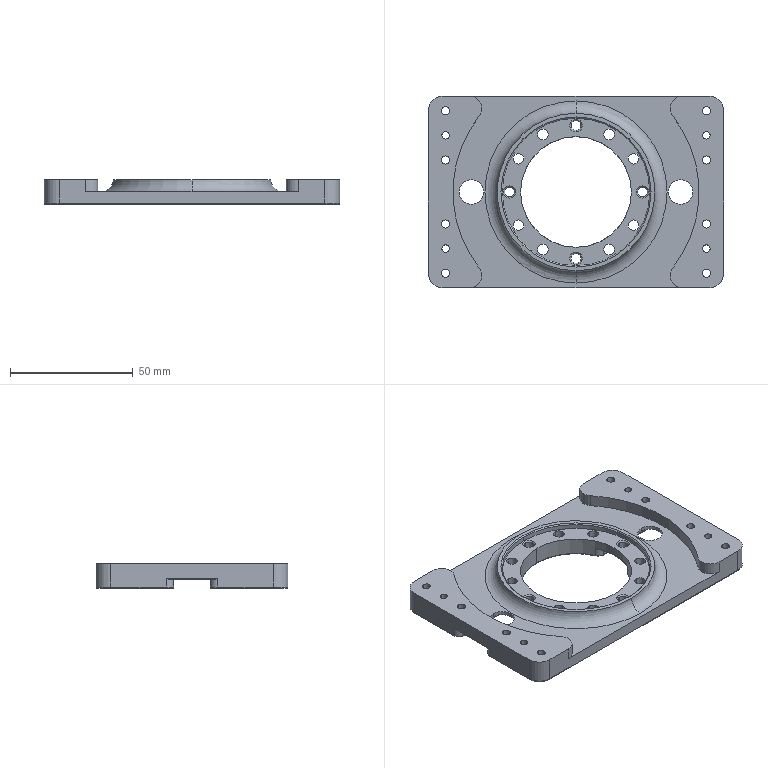NC program | NX | posted with a generic post | part box 120 x 78 x 10 mm
Lines 4596 to 5508 of 5508:
(ZLEVEL_PROFILE_1 , TOOL : D2R0.5)
N9082 T24 M6
N9084 G54
N9086 G17 G0 G90 X54.341 Y-39.568 B0. C0. S9500 M3
N9088 G43 Z30. H24
N9090 Z0.984
N9092 G94 G1 Z-0.016 F2500.
N9094 X54.173 Y-39.277
N9096 G3 X54. Y-39.177 R0.2
N9098 G1 X-54.
N9100 G2 X-60.177 Y-33. R6.177
N9102 G1 Y-10.5
N9104 G2 X-57. Y-7.323 R3.177
N9106 G1 X-23.238
N9108 G2 X-20.343 Y-9.192 R3.177
N9110 G3 X20.343 Y-9.192 R22.323
N9112 G2 X23.238 Y-7.323 R3.177
N9114 G1 X57.
N9116 G2 X60.177 Y-10.5 R3.177
N9118 G1 Y-33.
N9120 G2 X54. Y-39.177 R6.177
N9122 G1 Y-39.236 Z-0.028
N9124 Y-39.282 Z-0.041
N9126 G3 X60.282 Y-33. R6.282
N9128 G1 Y-10.5
N9130 G3 X57. Y-7.218 R3.282
N9132 G1 X23.238
N9134 G3 X20.247 Y-9.149 R3.282
N9136 G2 X-20.247 Y-9.149 R22.218
N9138 G3 X-23.238 Y-7.218 R3.282
N9140 G1 X-57.
N9142 G3 X-60.282 Y-10.5 R3.282
N9144 G1 Y-33.
N9146 G3 X-54. Y-39.282 R6.282
N9148 G1 X54.
N9150 Y-39.335 Z-0.058
N9152 Y-39.38 Z-0.075
N9154 X-54.
N9156 G2 X-60.38 Y-33. R6.38
N9158 G1 Y-10.5
N9160 G2 X-57. Y-7.12 R3.38
N9162 G1 X-23.238
N9164 G2 X-20.157 Y-9.108 R3.38
N9166 G3 X20.157 Y-9.108 R22.12
N9168 G2 X23.238 Y-7.12 R3.38
N9170 G1 X57.
N9172 G2 X60.38 Y-10.5 R3.38
N9174 G1 Y-33.
N9176 G2 X54. Y-39.38 R6.38
N9178 G1 Y-39.43 Z-0.097
N9180 Y-39.473 Z-0.119
N9182 G3 X60.473 Y-33. R6.473
N9184 G1 Y-10.5
N9186 G3 X57. Y-7.027 R3.473
N9188 G1 X23.238
N9190 G3 X20.073 Y-9.07 R3.473
N9192 G2 X-20.073 Y-9.07 R22.027
N9194 G3 X-23.238 Y-7.027 R3.473
N9196 G1 X-57.
N9198 G3 X-60.473 Y-10.5 R3.473
N9200 G1 Y-33.
N9202 G3 X-54. Y-39.473 R6.473
N9204 G1 X54.
N9206 Y-39.519 Z-0.145
N9208 Y-39.56 Z-0.171
N9210 X-54.
N9212 G2 X-60.56 Y-33. R6.56
N9214 G1 Y-10.5
N9216 G2 X-57. Y-6.94 R3.56
N9218 G1 X-23.238
N9220 G2 X-19.994 Y-9.034 R3.56
N9222 G3 X19.994 Y-9.034 R21.94
N9224 G2 X23.238 Y-6.94 R3.56
N9226 G1 X57.
N9228 G2 X60.56 Y-10.5 R3.56
N9230 G1 Y-33.
N9232 G2 X54. Y-39.56 R6.56
N9234 G1 Y-39.602 Z-0.202
N9236 Y-39.64 Z-0.232
N9238 G3 X60.64 Y-33. R6.64
N9240 G1 Y-10.5
N9242 G3 X57. Y-6.86 R3.64
N9244 G1 X23.238
N9246 G3 X19.92 Y-9.001 R3.64
N9248 G2 X-19.92 Y-9.001 R21.86
N9250 G3 X-23.238 Y-6.86 R3.64
N9252 G1 X-57.
N9254 G3 X-60.64 Y-10.5 R3.64
N9256 G1 Y-33.
N9258 G3 X-54. Y-39.64 R6.64
N9260 G1 X54.
N9262 Y-39.679 Z-0.266
N9264 Y-39.714 Z-0.3
N9266 X-54.
N9268 G2 X-60.714 Y-33. R6.714
N9270 G1 Y-10.5
N9272 G2 X-57. Y-6.786 R3.714
N9274 G1 X-23.238
N9276 G2 X-19.853 Y-8.971 R3.714
N9278 G3 X19.853 Y-8.971 R21.786
N9280 G2 X23.238 Y-6.786 R3.714
N9282 G1 X57.
N9284 G2 X60.714 Y-10.5 R3.714
N9286 G1 Y-33.
N9288 G2 X54. Y-39.714 R6.714
N9290 G1 Y-39.749 Z-0.338
N9292 Y-39.781 Z-0.376
N9294 G3 X60.781 Y-33. R6.781
N9296 G1 Y-10.5
N9298 G3 X57. Y-6.719 R3.781
N9300 G1 X23.238
N9302 G3 X19.792 Y-8.943 R3.781
N9304 G2 X-19.792 Y-8.943 R21.719
N9306 G3 X-23.238 Y-6.719 R3.781
N9308 G1 X-57.
N9310 G3 X-60.781 Y-10.5 R3.781
N9312 G1 Y-33.
N9314 G3 X-54. Y-39.781 R6.781
N9316 G1 X54.
N9318 Y-39.812 Z-0.416
N9320 Y-39.84 Z-0.457
N9322 X-54.
N9324 G2 X-60.84 Y-33. R6.84
N9326 G1 Y-10.5
N9328 G2 X-57. Y-6.66 R3.84
N9330 G1 X-23.238
N9332 G2 X-19.739 Y-8.919 R3.84
N9334 G3 X19.739 Y-8.919 R21.66
N9336 G2 X23.238 Y-6.66 R3.84
N9338 G1 X57.
N9340 G2 X60.84 Y-10.5 R3.84
N9342 G1 Y-33.
N9344 G2 X54. Y-39.84 R6.84
N9346 G1 Y-39.866 Z-0.501
N9348 Y-39.89 Z-0.544
N9350 G3 X60.89 Y-33. R6.89
N9352 G1 Y-10.5
N9354 G3 X57. Y-6.61 R3.89
N9356 G1 X23.238
N9358 G3 X19.693 Y-8.898 R3.89
N9360 G2 X-19.693 Y-8.898 R21.61
N9362 G3 X-23.238 Y-6.61 R3.89
N9364 G1 X-57.
N9366 G3 X-60.89 Y-10.5 R3.89
N9368 G1 Y-33.
N9370 G3 X-54. Y-39.89 R6.89
N9372 G1 X54.
N9374 Y-39.912 Z-0.59
N9376 Y-39.931 Z-0.635
N9378 X-54.
N9380 G2 X-60.931 Y-33. R6.931
N9382 G1 Y-10.5
N9384 G2 X-57. Y-6.569 R3.931
N9386 G1 X-23.238
N9388 G2 X-19.656 Y-8.881 R3.931
N9390 G3 X19.656 Y-8.881 R21.569
N9392 G2 X23.238 Y-6.569 R3.931
N9394 G1 X57.
N9396 G2 X60.931 Y-10.5 R3.931
N9398 G1 Y-33.
N9400 G2 X54. Y-39.931 R6.931
N9402 G1 Y-39.948 Z-0.681
N9404 Y-39.962 Z-0.726
N9406 G3 X60.962 Y-33. R6.962
N9408 G1 Y-10.5
N9410 G3 X57. Y-6.538 R3.962
N9412 G1 X23.238
N9414 G3 X19.627 Y-8.869 R3.962
N9416 G2 X-19.627 Y-8.869 R21.538
N9418 G3 X-23.238 Y-6.538 R3.962
N9420 G1 X-57.
N9422 G3 X-60.962 Y-10.5 R3.962
N9424 G1 Y-33.
N9426 G3 X-54. Y-39.962 R6.962
N9428 G1 X54.
N9430 Y-39.974 Z-0.772
N9432 Y-39.983 Z-0.818
N9434 X-54.
N9436 G2 X-60.983 Y-33. R6.983
N9438 G1 Y-10.5
N9440 G2 X-57. Y-6.517 R3.983
N9442 G1 X-23.238
N9444 G2 X-19.608 Y-8.86 R3.983
N9446 G3 X19.608 Y-8.86 R21.517
N9448 G2 X23.238 Y-6.517 R3.983
N9450 G1 X57.
N9452 G2 X60.983 Y-10.5 R3.983
N9454 G1 Y-33.
N9456 G2 X54. Y-39.983 R6.983
N9458 G1 Y-39.991 Z-0.863
N9460 Y-39.996 Z-0.909
N9462 G3 X60.996 Y-33. R6.996
N9464 G1 Y-10.5
N9466 G3 X57. Y-6.504 R3.996
N9468 G1 X23.238
N9470 G3 X19.597 Y-8.855 R3.996
N9472 G2 X-19.597 Y-8.855 R21.504
N9474 G3 X-23.238 Y-6.504 R3.996
N9476 G1 X-57.
N9478 G3 X-60.996 Y-10.5 R3.996
N9480 G1 Y-33.
N9482 G3 X-54. Y-39.996 R6.996
N9484 G1 X54.
N9486 Y-39.998 Z-1.
N9488 X-54.
N9490 G2 X-60.999 Y-33. R6.999
N9492 G1 Y-10.584
N9494 G2 X-57. Y-6.5 R4.002
N9496 G1 X-23.238
N9498 G2 X-19.593 Y-8.853 R4.004
N9500 G3 X19.569 Y-8.905 R21.501
N9502 G2 X23.238 Y-6.5 R4.008
N9504 G1 X56.994
N9506 G2 X61. Y-10.505 R4.005
N9508 G1 Y-32.924
N9510 G2 X54. Y-39.998 R7.
N9512 G3 X53.827 Y-40.098 R0.2
N9514 G1 X53.654 Y-40.398
N9516 Z0.
N9518 G0 Z30.
N9520 X-54.341 Y39.568
N9522 Z0.984
N9524 G1 Z-0.016
N9526 X-54.173 Y39.277
N9528 G3 X-54. Y39.177 R0.2
N9530 G1 X54.
N9532 G2 X60.177 Y33. R6.177
N9534 G1 Y10.5
N9536 G2 X57. Y7.323 R3.177
N9538 G1 X23.238
N9540 G2 X20.343 Y9.192 R3.177
N9542 G3 X-20.343 Y9.192 R22.323
N9544 G2 X-23.238 Y7.323 R3.177
N9546 G1 X-57.
N9548 G2 X-60.177 Y10.5 R3.177
N9550 G1 Y33.
N9552 G2 X-54. Y39.177 R6.177
N9554 G1 Y39.236 Z-0.028
N9556 Y39.282 Z-0.041
N9558 G3 X-60.282 Y33. R6.282
N9560 G1 Y10.5
N9562 G3 X-57. Y7.218 R3.282
N9564 G1 X-23.238
N9566 G3 X-20.247 Y9.149 R3.282
N9568 G2 X20.247 Y9.149 R22.218
N9570 G3 X23.238 Y7.218 R3.282
N9572 G1 X57.
N9574 G3 X60.282 Y10.5 R3.282
N9576 G1 Y33.
N9578 G3 X54. Y39.282 R6.282
N9580 G1 X-54.
N9582 Y39.335 Z-0.058
N9584 Y39.38 Z-0.075
N9586 X54.
N9588 G2 X60.38 Y33. R6.38
N9590 G1 Y10.5
N9592 G2 X57. Y7.12 R3.38
N9594 G1 X23.238
N9596 G2 X20.157 Y9.108 R3.38
N9598 G3 X-20.157 Y9.108 R22.12
N9600 G2 X-23.238 Y7.12 R3.38
N9602 G1 X-57.
N9604 G2 X-60.38 Y10.5 R3.38
N9606 G1 Y33.
N9608 G2 X-54. Y39.38 R6.38
N9610 G1 Y39.43 Z-0.097
N9612 Y39.473 Z-0.119
N9614 G3 X-60.473 Y33. R6.473
N9616 G1 Y10.5
N9618 G3 X-57. Y7.027 R3.473
N9620 G1 X-23.238
N9622 G3 X-20.073 Y9.07 R3.473
N9624 G2 X20.073 Y9.07 R22.027
N9626 G3 X23.238 Y7.027 R3.473
N9628 G1 X57.
N9630 G3 X60.473 Y10.5 R3.473
N9632 G1 Y33.
N9634 G3 X54. Y39.473 R6.473
N9636 G1 X-54.
N9638 Y39.519 Z-0.145
N9640 Y39.56 Z-0.171
N9642 X54.
N9644 G2 X60.56 Y33. R6.56
N9646 G1 Y10.5
N9648 G2 X57. Y6.94 R3.56
N9650 G1 X23.238
N9652 G2 X19.994 Y9.034 R3.56
N9654 G3 X-19.994 Y9.034 R21.94
N9656 G2 X-23.238 Y6.94 R3.56
N9658 G1 X-57.
N9660 G2 X-60.56 Y10.5 R3.56
N9662 G1 Y33.
N9664 G2 X-54. Y39.56 R6.56
N9666 G1 Y39.602 Z-0.202
N9668 Y39.64 Z-0.232
N9670 G3 X-60.64 Y33. R6.64
N9672 G1 Y10.5
N9674 G3 X-57. Y6.86 R3.64
N9676 G1 X-23.238
N9678 G3 X-19.92 Y9.001 R3.64
N9680 G2 X19.92 Y9.001 R21.86
N9682 G3 X23.238 Y6.86 R3.64
N9684 G1 X57.
N9686 G3 X60.64 Y10.5 R3.64
N9688 G1 Y33.
N9690 G3 X54. Y39.64 R6.64
N9692 G1 X-54.
N9694 Y39.679 Z-0.266
N9696 Y39.714 Z-0.3
N9698 X54.
N9700 G2 X60.714 Y33. R6.714
N9702 G1 Y10.5
N9704 G2 X57. Y6.786 R3.714
N9706 G1 X23.238
N9708 G2 X19.853 Y8.971 R3.714
N9710 G3 X-19.853 Y8.971 R21.786
N9712 G2 X-23.238 Y6.786 R3.714
N9714 G1 X-57.
N9716 G2 X-60.714 Y10.5 R3.714
N9718 G1 Y33.
N9720 G2 X-54. Y39.714 R6.714
N9722 G1 Y39.749 Z-0.338
N9724 Y39.781 Z-0.376
N9726 G3 X-60.781 Y33. R6.781
N9728 G1 Y10.5
N9730 G3 X-57. Y6.719 R3.781
N9732 G1 X-23.238
N9734 G3 X-19.792 Y8.943 R3.781
N9736 G2 X19.792 Y8.943 R21.719
N9738 G3 X23.238 Y6.719 R3.781
N9740 G1 X57.
N9742 G3 X60.781 Y10.5 R3.781
N9744 G1 Y33.
N9746 G3 X54. Y39.781 R6.781
N9748 G1 X-54.
N9750 Y39.812 Z-0.416
N9752 Y39.84 Z-0.457
N9754 X54.
N9756 G2 X60.84 Y33. R6.84
N9758 G1 Y10.5
N9760 G2 X57. Y6.66 R3.84
N9762 G1 X23.238
N9764 G2 X19.739 Y8.919 R3.84
N9766 G3 X-19.739 Y8.919 R21.66
N9768 G2 X-23.238 Y6.66 R3.84
N9770 G1 X-57.
N9772 G2 X-60.84 Y10.5 R3.84
N9774 G1 Y33.
N9776 G2 X-54. Y39.84 R6.84
N9778 G1 Y39.866 Z-0.501
N9780 Y39.89 Z-0.544
N9782 G3 X-60.89 Y33. R6.89
N9784 G1 Y10.5
N9786 G3 X-57. Y6.61 R3.89
N9788 G1 X-23.238
N9790 G3 X-19.693 Y8.898 R3.89
N9792 G2 X19.693 Y8.898 R21.61
N9794 G3 X23.238 Y6.61 R3.89
N9796 G1 X57.
N9798 G3 X60.89 Y10.5 R3.89
N9800 G1 Y33.
N9802 G3 X54. Y39.89 R6.89
N9804 G1 X-54.
N9806 Y39.912 Z-0.59
N9808 Y39.931 Z-0.635
N9810 X54.
N9812 G2 X60.931 Y33. R6.931
N9814 G1 Y10.5
N9816 G2 X57. Y6.569 R3.931
N9818 G1 X23.238
N9820 G2 X19.656 Y8.881 R3.931
N9822 G3 X-19.656 Y8.881 R21.569
N9824 G2 X-23.238 Y6.569 R3.931
N9826 G1 X-57.
N9828 G2 X-60.931 Y10.5 R3.931
N9830 G1 Y33.
N9832 G2 X-54. Y39.931 R6.931
N9834 G1 Y39.948 Z-0.681
N9836 Y39.962 Z-0.726
N9838 G3 X-60.962 Y33. R6.962
N9840 G1 Y10.5
N9842 G3 X-57. Y6.538 R3.962
N9844 G1 X-23.238
N9846 G3 X-19.627 Y8.869 R3.962
N9848 G2 X19.627 Y8.869 R21.538
N9850 G3 X23.238 Y6.538 R3.962
N9852 G1 X57.
N9854 G3 X60.962 Y10.5 R3.962
N9856 G1 Y33.
N9858 G3 X54. Y39.962 R6.962
N9860 G1 X-54.
N9862 Y39.974 Z-0.772
N9864 Y39.983 Z-0.818
N9866 X54.
N9868 G2 X60.983 Y33. R6.983
N9870 G1 Y10.5
N9872 G2 X57. Y6.517 R3.983
N9874 G1 X23.238
N9876 G2 X19.608 Y8.86 R3.983
N9878 G3 X-19.608 Y8.86 R21.517
N9880 G2 X-23.238 Y6.517 R3.983
N9882 G1 X-57.
N9884 G2 X-60.983 Y10.5 R3.983
N9886 G1 Y33.
N9888 G2 X-54. Y39.983 R6.983
N9890 G1 Y39.991 Z-0.863
N9892 Y39.996 Z-0.909
N9894 G3 X-60.996 Y33. R6.996
N9896 G1 Y10.5
N9898 G3 X-57. Y6.504 R3.996
N9900 G1 X-23.238
N9902 G3 X-19.597 Y8.854 R3.996
N9904 G2 X19.597 Y8.855 R21.504
N9906 G3 X23.238 Y6.504 R3.996
N9908 G1 X57.
N9910 G3 X60.996 Y10.5 R3.996
N9912 G1 Y33.
N9914 G3 X54. Y39.996 R6.996
N9916 G1 X-54.
N9918 Y40. Z-1.
N9920 X54.
N9922 G2 X61. Y33. R7.001
N9924 G1 Y10.584
N9926 G2 X57. Y6.5 R4.004
N9928 G1 X23.238
N9930 G2 X19.569 Y8.907 R4.005
N9932 G3 X-19.569 Y8.907 R21.502
N9934 G2 X-23.238 Y6.5 R4.005
N9936 G1 X-57.
N9938 G2 X-60.999 Y10.5 R4.001
N9940 G1 Y32.924
N9942 G2 X-54. Y40. R7.002
N9944 G3 X-53.827 Y40.1 R0.2
N9946 G1 X-53.654 Y40.4
N9948 Z0.
N9950 G0 Z30.
(ZLEVEL_PROFILE_1_COPY , TOOL : D2R0.5)
N9952 X60.694 Y8.109
N9954 Z-2.616
N9956 G1 Z-3.616
N9958 X60.365 Y8.152
N9960 G3 X60.181 Y8.075 R0.2
N9962 G1 Y-8.075
N9964 X60.239 Y-8.147 Z-3.629
N9966 X60.286 Y-8.219 Z-3.642
N9968 Y8.219
N9970 X60.339 Y8.293 Z-3.659
N9972 X60.384 Y8.367 Z-3.677
N9974 Y-8.367
N9976 X60.433 Y-8.444 Z-3.699
N9978 X60.476 Y-8.521 Z-3.721
N9980 Y8.521
N9982 X60.522 Y8.601 Z-3.747
N9984 X60.563 Y8.682 Z-3.773
N9986 Y-8.682
N9988 X60.605 Y-8.765 Z-3.804
N9990 X60.643 Y-8.849 Z-3.834
N9992 Y8.849
N9994 X60.682 Y8.936 Z-3.869
N9996 X60.717 Y9.023 Z-3.903
N9998 Y-9.023
N10000 X60.752 Y-9.112 Z-3.941
N10002 X60.783 Y-9.202 Z-3.979
N10004 Y9.202
N10006 X60.814 Y9.294 Z-4.019
N10008 X60.842 Y9.386 Z-4.06
N10010 Y-9.386
N10012 X60.868 Y-9.481 Z-4.104
N10014 X60.892 Y-9.575 Z-4.147
N10016 Y9.575
N10018 X60.913 Y9.672 Z-4.193
N10020 X60.932 Y9.768 Z-4.239
N10022 Y-9.768
N10024 X60.949 Y-9.861 Z-4.284
N10026 X60.963 Y-9.954 Z-4.329
N10028 Y9.954
N10030 X60.974 Y10.046 Z-4.374
N10032 X60.984 Y10.138 Z-4.419
N10034 Y-10.138
N10036 X60.991 Y-10.236 Z-4.425
N10038 X60.997 Y-10.335 Z-4.431
N10040 X60.999 Y-10.433 Z-4.436
N10042 X61. Y-10.532 Z-4.442
N10044 Y-10.631 Z-4.448
N10046 Y-10.729 Z-4.453
N10048 X60.999 Y-10.828 Z-4.459
N10050 Y-10.926 Z-4.465
N10052 Y-11.025 Z-4.47
N10054 Y-11.123 Z-4.476
N10056 Y-11.222 Z-4.481
N10058 Y-11.321 Z-4.487
N10060 Y-11.419 Z-4.493
N10062 Y-11.518 Z-4.498
N10064 Y-11.616 Z-4.504
N10066 X60.997 Y-11.715 Z-4.51
N10068 X60.999 Y-11.609
N10070 Y-10.419
N10072 X60.996 Y-10.39
N10074 Y10.319
N10076 X60.999 Y10.418 Z-4.515
N10078 X61. Y10.518 Z-4.52
N10080 Y11.312 Z-4.563
N10082 Y11.411 Z-4.568
N10084 Y11.51 Z-4.573
N10086 Y11.609 Z-4.579
N10088 Y11.708 Z-4.584
N10090 Y11.808 Z-4.589
N10092 Y11.907 Z-4.595
N10094 Y12.006 Z-4.6
N10096 Y-12.006
N10098 G3 X61.1 Y-12.179 R0.2
N10100 G1 X61.4 Y-12.353
N10102 Z-3.6
N10104 G0 Z30.
N10106 X20.677 Y-6.922
N10108 Z-2.616
N10110 G1 Z-3.616
N10112 X20.967 Y-7.082
N10114 G3 X21.167 Y-7.078 R0.2
N10116 X21.167 Y7.078 R22.319
N10118 G1 X21.091 Y7.12 Z-3.629
N10120 X21.026 Y7.167 Z-3.642
N10122 G2 X21.026 Y-7.167 R22.214
N10124 G1 X20.955 Y-7.213 Z-3.659
N10126 X20.89 Y-7.262 Z-3.677
N10128 G3 X20.89 Y7.262 R22.116
N10130 G1 X20.821 Y7.311 Z-3.699
N10132 X20.757 Y7.362 Z-3.721
N10134 G2 X20.757 Y-7.362 R22.024
N10136 G1 X20.689 Y-7.416 Z-3.747
N10138 X20.626 Y-7.471 Z-3.773
N10140 G3 X20.626 Y7.471 R21.937
N10142 G1 X20.56 Y7.527 Z-3.804
N10144 X20.498 Y7.586 Z-3.834
N10146 G2 X20.498 Y-7.586 R21.857
N10148 G1 X20.434 Y-7.646 Z-3.869
N10150 X20.374 Y-7.708 Z-3.903
N10152 G3 X20.374 Y7.708 R21.783
N10154 G1 X20.312 Y7.772 Z-3.941
N10156 X20.253 Y7.837 Z-3.979
N10158 G2 X20.253 Y-7.837 R21.717
N10160 G1 X20.194 Y-7.905 Z-4.019
N10162 X20.137 Y-7.973 Z-4.06
N10164 G3 X20.137 Y7.973 R21.658
N10166 G1 X20.081 Y8.044 Z-4.104
N10168 X20.027 Y8.115 Z-4.147
N10170 G2 X20.027 Y-8.115 R21.608
N10172 G1 X19.973 Y-8.189 Z-4.193
N10174 X19.922 Y-8.263 Z-4.239
N10176 G3 X19.922 Y8.263 R21.568
N10178 G1 X19.874 Y8.336 Z-4.284
N10180 X19.828 Y8.409 Z-4.329
N10182 G2 X19.828 Y-8.409 R21.537
N10184 G1 X19.784 Y-8.482 Z-4.374
N10186 X19.742 Y-8.555 Z-4.419
N10188 G3 X19.742 Y8.555 R21.516
N10190 G1 X19.696 Y8.642 Z-4.425
N10192 X19.651 Y8.73 Z-4.431
N10194 X19.608 Y8.819 Z-4.436
N10196 X19.568 Y8.908 Z-4.442
N10198 X19.527 Y8.998 Z-4.448
N10200 X19.485 Y9.087 Z-4.453
N10202 X19.444 Y9.176 Z-4.459
N10204 X19.401 Y9.265 Z-4.465
N10206 X19.359 Y9.354 Z-4.47
N10208 X19.316 Y9.442 Z-4.476
N10210 X19.272 Y9.53 Z-4.481
N10212 X19.228 Y9.619 Z-4.487
N10214 X19.184 Y9.707 Z-4.493
N10216 X19.14 Y9.794 Z-4.498
N10218 X19.095 Y9.882 Z-4.504
N10220 X19.049 Y9.969 Z-4.51
N10222 G2 X19.637 Y8.765 R21.502
N10224 X19.637 Y-8.765 R21.504
N10226 G1 X19.602 Y-8.835
N10228 X19.421 Y-9.226
N10230 X19.382 Y-9.31 Z-4.52
N10232 X19.34 Y-9.392 Z-4.53
N10234 X19.3 Y-9.475 Z-4.54
N10236 X19.259 Y-9.558 Z-4.55
N10238 X19.218 Y-9.64 Z-4.56
N10240 X19.176 Y-9.723 Z-4.57
N10242 X19.134 Y-9.805 Z-4.58
N10244 X19.092 Y-9.887 Z-4.59
N10246 X19.049 Y-9.969 Z-4.6
N10248 G3 X19.049 Y9.969 R21.5
N10250 X18.88 Y10.076 R0.2
N10252 G1 X18.531 Y10.091
N10254 Z-3.6
N10256 G0 Z30.
N10258 X-20.677 Y6.922
N10260 Z-2.616
N10262 G1 Z-3.616
N10264 X-20.967 Y7.082
N10266 G3 X-21.167 Y7.078 R0.2
N10268 X-21.167 Y-7.078 R22.319
N10270 G1 X-21.091 Y-7.12 Z-3.629
N10272 X-21.026 Y-7.167 Z-3.642
N10274 G2 X-21.026 Y7.167 R22.214
N10276 G1 X-20.955 Y7.213 Z-3.659
N10278 X-20.89 Y7.262 Z-3.677
N10280 G3 X-20.89 Y-7.262 R22.116
N10282 G1 X-20.821 Y-7.311 Z-3.699
N10284 X-20.757 Y-7.362 Z-3.721
N10286 G2 X-20.757 Y7.362 R22.024
N10288 G1 X-20.689 Y7.416 Z-3.747
N10290 X-20.626 Y7.471 Z-3.773
N10292 G3 X-20.626 Y-7.471 R21.937
N10294 G1 X-20.56 Y-7.527 Z-3.804
N10296 X-20.498 Y-7.586 Z-3.834
N10298 G2 X-20.498 Y7.586 R21.857
N10300 G1 X-20.434 Y7.646 Z-3.869
N10302 X-20.374 Y7.708 Z-3.903
N10304 G3 X-20.374 Y-7.708 R21.783
N10306 G1 X-20.312 Y-7.772 Z-3.941
N10308 X-20.253 Y-7.837 Z-3.979
N10310 G2 X-20.253 Y7.837 R21.717
N10312 G1 X-20.194 Y7.905 Z-4.019
N10314 X-20.137 Y7.973 Z-4.06
N10316 G3 X-20.137 Y-7.973 R21.658
N10318 G1 X-20.081 Y-8.044 Z-4.104
N10320 X-20.027 Y-8.115 Z-4.147
N10322 G2 X-20.027 Y8.115 R21.608
N10324 G1 X-19.973 Y8.189 Z-4.193
N10326 X-19.922 Y8.263 Z-4.239
N10328 G3 X-19.922 Y-8.263 R21.568
N10330 G1 X-19.874 Y-8.336 Z-4.284
N10332 X-19.828 Y-8.409 Z-4.329
N10334 G2 X-19.828 Y8.409 R21.537
N10336 G1 X-19.784 Y8.482 Z-4.374
N10338 X-19.742 Y8.555 Z-4.419
N10340 G3 X-19.742 Y-8.555 R21.516
N10342 G1 X-19.696 Y-8.642 Z-4.425
N10344 X-19.651 Y-8.73 Z-4.431
N10346 X-19.608 Y-8.819 Z-4.436
N10348 X-19.568 Y-8.908 Z-4.442
N10350 X-19.527 Y-8.998 Z-4.448
N10352 X-19.485 Y-9.087 Z-4.453
N10354 X-19.443 Y-9.176 Z-4.459
N10356 X-19.401 Y-9.265 Z-4.465
N10358 X-19.359 Y-9.354 Z-4.47
N10360 X-19.316 Y-9.442 Z-4.476
N10362 X-19.272 Y-9.531 Z-4.481
N10364 X-19.228 Y-9.619 Z-4.487
N10366 X-19.184 Y-9.707 Z-4.493
N10368 X-19.139 Y-9.795 Z-4.498
N10370 X-19.094 Y-9.882 Z-4.504
N10372 X-19.049 Y-9.97 Z-4.51
N10374 G2 X-19.637 Y-8.765 R24.584
N10376 X-19.637 Y8.765 R21.504
N10378 G1 X-19.595 Y8.848
N10380 X-19.422 Y9.228
N10382 X-19.38 Y9.31 Z-4.52
N10384 X-19.34 Y9.393 Z-4.53
N10386 X-19.299 Y9.476 Z-4.54
N10388 X-19.258 Y9.559 Z-4.55
N10390 X-19.217 Y9.641 Z-4.56
N10392 X-19.176 Y9.724 Z-4.57
N10394 X-19.134 Y9.806 Z-4.58
N10396 X-19.091 Y9.888 Z-4.59
N10398 X-19.049 Y9.97 Z-4.6
N10400 G3 X-19.049 Y-9.97 R21.519
N10402 X-18.88 Y-10.077 R0.2
N10404 G1 X-18.53 Y-10.091
N10406 Z-3.6
N10408 G0 Z30.
N10410 X-60.694 Y-8.109
N10412 Z-2.616
N10414 G1 Z-3.616
N10416 X-60.365 Y-8.152
N10418 G3 X-60.181 Y-8.075 R0.2
N10420 G1 Y8.075
N10422 X-60.239 Y8.147 Z-3.629
N10424 X-60.286 Y8.219 Z-3.642
N10426 Y-8.219
N10428 X-60.339 Y-8.293 Z-3.659
N10430 X-60.384 Y-8.367 Z-3.677
N10432 Y8.367
N10434 X-60.433 Y8.444 Z-3.699
N10436 X-60.476 Y8.521 Z-3.721
N10438 Y-8.521
N10440 X-60.522 Y-8.601 Z-3.747
N10442 X-60.563 Y-8.682 Z-3.773
N10444 Y8.682
N10446 X-60.605 Y8.765 Z-3.804
N10448 X-60.643 Y8.849 Z-3.834
N10450 Y-8.849
N10452 X-60.682 Y-8.936 Z-3.869
N10454 X-60.717 Y-9.023 Z-3.903
N10456 Y9.023
N10458 X-60.752 Y9.112 Z-3.941
N10460 X-60.783 Y9.202 Z-3.979
N10462 Y-9.202
N10464 X-60.814 Y-9.294 Z-4.019
N10466 X-60.842 Y-9.386 Z-4.06
N10468 Y9.386
N10470 X-60.868 Y9.481 Z-4.104
N10472 X-60.892 Y9.575 Z-4.147
N10474 Y-9.575
N10476 X-60.913 Y-9.672 Z-4.193
N10478 X-60.932 Y-9.768 Z-4.239
N10480 Y9.768
N10482 X-60.949 Y9.861 Z-4.284
N10484 X-60.963 Y9.954 Z-4.329
N10486 Y-9.954
N10488 X-60.974 Y-10.046 Z-4.374
N10490 X-60.984 Y-10.138 Z-4.419
N10492 Y10.138
N10494 X-60.991 Y10.236 Z-4.425
N10496 X-60.997 Y10.335 Z-4.431
N10498 X-60.999 Y10.433 Z-4.436
N10500 X-61. Y10.532 Z-4.442
N10502 Y10.729 Z-4.453
N10504 Y10.828 Z-4.459
N10506 Y10.926 Z-4.465
N10508 Y11.025 Z-4.47
N10510 Y11.123 Z-4.476
N10512 Y11.222 Z-4.481
N10514 Y11.32 Z-4.487
N10516 Y11.419 Z-4.493
N10518 Y11.518 Z-4.498
N10520 Y11.616 Z-4.504
N10522 X-60.997 Y11.715 Z-4.51
N10524 Y10.419
N10526 X-60.996 Y10.39
N10528 Y-10.39
N10530 X-61. Y-10.485 Z-4.515
N10532 Y-10.58 Z-4.52
N10534 Y-11.341 Z-4.563
N10536 X-60.999 Y-11.436 Z-4.568
N10538 Y-11.531 Z-4.573
N10540 X-61. Y-11.626 Z-4.579
N10542 Y-11.721 Z-4.584
N10544 Y-11.816 Z-4.589
N10546 Y-11.911 Z-4.595
N10548 Y-12.006 Z-4.6
N10550 Y12.006
N10552 G3 X-61.1 Y12.179 R0.2
N10554 G1 X-61.4 Y12.353
N10556 Z-3.6
N10558 G0 Z30.
N10560 M5
(刀补17 , TOOL : D3)
N10562 T17 M6
N10564 G54
N10566 G17 G0 G90 X-53. Y23. B0. C0. S9500 M3
N10568 G43 Z30. H17
N10570 Z0.5
N10572 G41 G94 G1 X-53.027 Y23.096 F1250. D17
N10574 G3 X-53.45 Y23. R0.222
N10576 X-53.45 Y23. Z-2. I0.45 J0.
N10578 X-53.139 Y23.428 Z-4. R-0.45
N10580 X-53.428 Y22.861 R0.45
N10582 X-53.139 Y23.428 R-0.45
N10584 X-53.1 Y22.996 R0.222
N10586 G40
N10588 G1 X-53. Y23.
N10590 G0 Z30.
N10592 Y-23.
N10594 Z0.5
N10596 G41 G1 X-53.027 Y-22.904
N10598 G3 X-53.45 Y-23. R0.222
N10600 X-53.45 Y-23. Z-2. I0.45 J0.
N10602 X-53.139 Y-22.572 Z-4. R-0.45
N10604 X-53.428 Y-23.139 R0.45
N10606 X-53.139 Y-22.572 R-0.45
N10608 X-53.1 Y-23.004 R0.222
N10610 G40
N10612 G1 X-53. Y-23.
N10614 G0 Z30.
N10616 X-27. Y0.
N10618 Z-3.1
N10620 G41 G1 X-27.027 Y0.096
N10622 G3 X-27.45 Y0. R0.222
N10624 X-27.45 Y0. Z-5.6 I0.45 J0.
N10626 X-27.139 Y0.428 Z-7.6 R-0.45
N10628 X-27.428 Y-0.139 R0.45
N10630 X-27.139 Y0.428 R-0.45
N10632 X-27.1 Y-0.004 R0.222
N10634 G40
N10636 G1 X-27. Y0.
N10638 G0 Z30.
N10640 X0. Y27.
N10642 Z0.5
N10644 G41 G1 X-0.027 Y27.096
N10646 G3 X-0.45 Y27. R0.222
N10648 X-0.45 Y27. Z-2. I0.45 J0.
N10650 X-0.45 Y27. Z-4.5 I0.45 J0.
N10652 X-0.45 Y27. Z-7. I0.45 J0.
N10654 X-0.028 Y26.551 Z-7.6 R0.45
N10656 X0.449 Y26.972 R0.45
N10658 X-0.028 Y26.551 R-0.45
N10660 X0.094 Y26.967 R0.222
N10662 G40
N10664 G1 X0. Y27.
N10666 G0 Z30.
N10668 X27. Y0.
N10670 Z-3.1
N10672 G41 G1 X26.973 Y0.096
N10674 G3 X26.55 Y0. R0.222
N10676 X26.55 Y0. Z-5.6 I0.45 J0.
N10678 X26.861 Y0.428 Z-7.6 R-0.45
N10680 X26.572 Y-0.139 R0.45
N10682 X26.861 Y0.428 R-0.45
N10684 X26.9 Y-0.004 R0.222
N10686 G40
N10688 G1 X27. Y0.
N10690 G0 Z30.
N10692 X53. Y23.
N10694 Z0.5
N10696 G41 G1 X52.973 Y23.096
N10698 G3 X52.55 Y23. R0.222
N10700 X52.55 Y23. Z-2. I0.45 J0.
N10702 X52.861 Y23.428 Z-4. R-0.45
N10704 X52.572 Y22.861 R0.45
N10706 X52.861 Y23.428 R-0.45
N10708 X52.9 Y22.996 R0.222
N10710 G40
N10712 G1 X53. Y23.
N10714 G0 Z30.
N10716 Y-23.
N10718 Z0.5
N10720 G41 G1 X52.973 Y-22.904
N10722 G3 X52.55 Y-23. R0.222
N10724 X52.55 Y-23. Z-2. I0.45 J0.
N10726 X52.861 Y-22.572 Z-4. R-0.45
N10728 X52.572 Y-23.139 R0.45
N10730 X52.861 Y-22.572 R-0.45
N10732 X52.9 Y-23.004 R0.222
N10734 G40
N10736 G1 X53. Y-23.
N10738 G0 Z30.
N10740 X0. Y-27.
N10742 Z0.5
N10744 G41 G1 X-0.027 Y-26.904
N10746 G3 X-0.45 Y-27. R0.222
N10748 X-0.45 Y-27. Z-2. I0.45 J0.
N10750 X-0.45 Y-27. Z-4.5 I0.45 J0.
N10752 X-0.45 Y-27. Z-7. I0.45 J0.
N10754 X-0.028 Y-27.449 Z-7.6 R0.45
N10756 X0.449 Y-27.028 R0.45
N10758 X-0.028 Y-27.449 R-0.45
N10760 X0.094 Y-27.033 R0.222
N10762 G40
N10764 G1 X0. Y-27.
N10766 G0 Z30.
N10768 M5
(刀补18 , TOOL : D2)
N10770 T18 M6
N10772 G54
N10774 G17 G0 G90 X-53. Y23. B0. C0. S9500 M3
N10776 G43 Z30. H18
N10778 Z-3.5
N10780 G41 G94 G1 X-53.027 Y23.096 F1250. D18
N10782 G3 X-53.45 Y23. R0.222
N10784 X-53.45 Y23. Z-6. I0.45 J0.
N10786 X-53.45 Y23. Z-8.5 I0.45 J0.
N10788 X-52.636 Y23.265 Z-10. R-0.45
N10790 X-53.265 Y23.364 R0.45
N10792 X-52.636 Y23.265 R-0.45
N10794 X-53.035 Y23.094 R0.222
N10796 G40
N10798 G1 X-53. Y23.
N10800 G0 Z30.
N10802 Y-23.
N10804 Z-3.5
N10806 G41 G1 X-53.027 Y-22.904
N10808 G3 X-53.45 Y-23. R0.222
N10810 X-53.45 Y-23. Z-6. I0.45 J0.
N10812 X-53.45 Y-23. Z-8.5 I0.45 J0.
N10814 X-52.636 Y-22.735 Z-10. R-0.45
N10816 X-53.265 Y-22.636 R0.45
N10818 X-52.636 Y-22.735 R-0.45
N10820 X-53.035 Y-22.906 R0.222
N10822 G40
N10824 G1 X-53. Y-23.
N10826 G0 Z30.
N10828 X53.
N10830 Z-3.5
N10832 G41 G1 X52.973 Y-22.904
N10834 G3 X52.55 Y-23. R0.222
N10836 X52.55 Y-23. Z-6. I0.45 J0.
N10838 X52.55 Y-23. Z-8.5 I0.45 J0.
N10840 X53.364 Y-22.735 Z-10. R-0.45
N10842 X52.735 Y-22.636 R0.45
N10844 X53.364 Y-22.735 R-0.45
N10846 X52.965 Y-22.906 R0.222
N10848 G40
N10850 G1 X53. Y-23.
N10852 G0 Z30.
N10854 Y23.
N10856 Z-3.5
N10858 G41 G1 X52.973 Y23.096
N10860 G3 X52.55 Y23. R0.222
N10862 X52.55 Y23. Z-6. I0.45 J0.
N10864 X52.55 Y23. Z-8.5 I0.45 J0.
N10866 X53.364 Y23.265 Z-10. R-0.45
N10868 X52.735 Y23.364 R0.45
N10870 X53.364 Y23.265 R-0.45
N10872 X52.965 Y23.094 R0.222
N10874 G40
N10876 G1 X53. Y23.
N10878 G0 Z30.
N10880 M5
N10882 M2